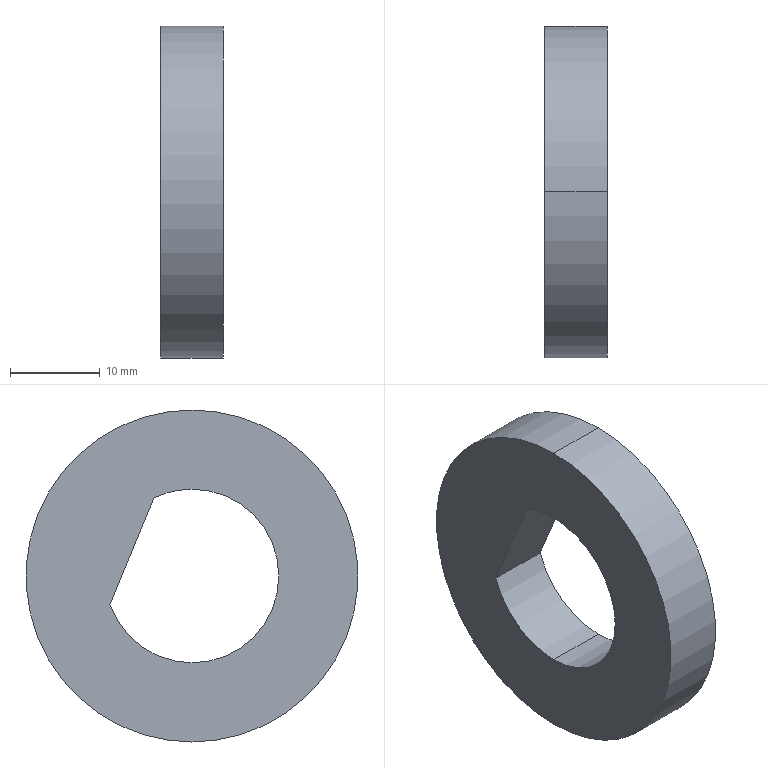Part | STEP file | Previa 01.sldasm-Part-11_Valor predeterminado | 1 solid | 8 faces | box 7 x 37.038 x 37.038 mm | volume 5630 mm3 | cylinder 5 | plane 3 | commonest cylinder face diameters 19.36 x3 37.038 x2
STEP:
#1=CARTESIAN_POINT('',(0.,0.,0.));
#2=DIRECTION('',(0.,0.,1.));
#3=DIRECTION('',(1.,0.,0.));
#4=AXIS2_PLACEMENT_3D('',#1,#2,#3);
#5=CARTESIAN_POINT('',(5.341,0.,-9.68));
#6=VERTEX_POINT('',#5);
#7=CARTESIAN_POINT('',(12.341,0.,-9.68));
#8=VERTEX_POINT('',#7);
#9=CARTESIAN_POINT('',(5.341,0.,-9.68));
#10=DIRECTION('',(1.,0.,0.));
#11=VECTOR('',#10,1.);
#12=LINE('',#9,#11);
#13=CARTESIAN_POINT('',(5.341,0.,0.));
#14=DIRECTION('',(1.,0.,0.));
#15=DIRECTION('',(0.,0.,-1.));
#16=AXIS2_PLACEMENT_3D('',#13,#14,#15);
#17=CYLINDRICAL_SURFACE('',#16,9.68);
#18=CARTESIAN_POINT('',(6.283,0.));
#19=DIRECTION('',(0.,1.));
#20=VECTOR('',#19,1.);
#21=LINE('',#18,#20);
#22=(GEOMETRIC_REPRESENTATION_CONTEXT(2)PARAMETRIC_REPRESENTATION_CONTEXT()REPRESENTATION_CONTEXT('',''));
#23=DEFINITIONAL_REPRESENTATION('',(#21),#22);
#24=PCURVE('',#17,#23);
#25=CARTESIAN_POINT('',(5.341,0.,0.));
#26=DIRECTION('',(1.,0.,0.));
#27=DIRECTION('',(0.,0.,-1.));
#28=AXIS2_PLACEMENT_3D('',#25,#26,#27);
#29=CYLINDRICAL_SURFACE('',#28,9.68);
#30=CARTESIAN_POINT('',(0.,0.));
#31=DIRECTION('',(0.,1.));
#32=VECTOR('',#31,1.);
#33=LINE('',#30,#32);
#34=(GEOMETRIC_REPRESENTATION_CONTEXT(2)PARAMETRIC_REPRESENTATION_CONTEXT()REPRESENTATION_CONTEXT('',''));
#35=DEFINITIONAL_REPRESENTATION('',(#33),#34);
#36=PCURVE('',#29,#35);
#37=SURFACE_CURVE('',#12,(#24,#36),.PCURVE_S1.);
#38=EDGE_CURVE('',#6,#8,#37,.T.);
#39=ORIENTED_EDGE('',*,*,#38,.T.);
#40=CARTESIAN_POINT('',(12.341,0.,9.68));
#41=VERTEX_POINT('',#40);
#42=CARTESIAN_POINT('',(12.341,0.,0.));
#43=DIRECTION('',(-1.,0.,0.));
#44=DIRECTION('',(0.,0.,-1.));
#45=AXIS2_PLACEMENT_3D('',#42,#43,#44);
#46=CIRCLE('',#45,9.68);
#47=CARTESIAN_POINT('',(6.283,7.));
#48=DIRECTION('',(-1.,0.));
#49=VECTOR('',#48,1.);
#50=LINE('',#47,#49);
#51=(GEOMETRIC_REPRESENTATION_CONTEXT(2)PARAMETRIC_REPRESENTATION_CONTEXT()REPRESENTATION_CONTEXT('',''));
#52=DEFINITIONAL_REPRESENTATION('',(#50),#51);
#53=PCURVE('',#17,#52);
#54=CARTESIAN_POINT('',(12.341,0.,0.));
#55=DIRECTION('',(-1.,0.,0.));
#56=DIRECTION('',(0.,0.,1.));
#57=AXIS2_PLACEMENT_3D('',#54,#55,#56);
#58=PLANE('',#57);
#59=CARTESIAN_POINT('',(0.,0.));
#60=DIRECTION('',(-1.,0.));
#61=AXIS2_PLACEMENT_2D('',#59,#60);
#62=CIRCLE('',#61,9.68);
#63=(GEOMETRIC_REPRESENTATION_CONTEXT(2)PARAMETRIC_REPRESENTATION_CONTEXT()REPRESENTATION_CONTEXT('',''));
#64=DEFINITIONAL_REPRESENTATION('',(#62),#63);
#65=PCURVE('',#58,#64);
#66=SURFACE_CURVE('',#46,(#53,#65),.PCURVE_S1.);
#67=EDGE_CURVE('',#8,#41,#66,.T.);
#68=ORIENTED_EDGE('',*,*,#67,.T.);
#69=CARTESIAN_POINT('',(5.341,0.,9.68));
#70=VERTEX_POINT('',#69);
#71=CARTESIAN_POINT('',(5.341,0.,9.68));
#72=DIRECTION('',(1.,0.,0.));
#73=VECTOR('',#72,1.);
#74=LINE('',#71,#73);
#75=CARTESIAN_POINT('',(3.142,0.));
#76=DIRECTION('',(0.,1.));
#77=VECTOR('',#76,1.);
#78=LINE('',#75,#77);
#79=(GEOMETRIC_REPRESENTATION_CONTEXT(2)PARAMETRIC_REPRESENTATION_CONTEXT()REPRESENTATION_CONTEXT('',''));
#80=DEFINITIONAL_REPRESENTATION('',(#78),#79);
#81=PCURVE('',#17,#80);
#82=CARTESIAN_POINT('',(5.341,0.,0.));
#83=DIRECTION('',(1.,0.,0.));
#84=DIRECTION('',(0.,0.,-1.));
#85=AXIS2_PLACEMENT_3D('',#82,#83,#84);
#86=CYLINDRICAL_SURFACE('',#85,9.68);
#87=CARTESIAN_POINT('',(3.142,0.));
#88=DIRECTION('',(0.,1.));
#89=VECTOR('',#88,1.);
#90=LINE('',#87,#89);
#91=(GEOMETRIC_REPRESENTATION_CONTEXT(2)PARAMETRIC_REPRESENTATION_CONTEXT()REPRESENTATION_CONTEXT('',''));
#92=DEFINITIONAL_REPRESENTATION('',(#90),#91);
#93=PCURVE('',#86,#92);
#94=SURFACE_CURVE('',#74,(#81,#93),.PCURVE_S1.);
#95=EDGE_CURVE('',#70,#41,#94,.T.);
#96=ORIENTED_EDGE('',*,*,#95,.F.);
#97=CARTESIAN_POINT('',(5.341,0.,0.));
#98=DIRECTION('',(-1.,0.,0.));
#99=DIRECTION('',(0.,0.,-1.));
#100=AXIS2_PLACEMENT_3D('',#97,#98,#99);
#101=CIRCLE('',#100,9.68);
#102=CARTESIAN_POINT('',(6.283,0.));
#103=DIRECTION('',(-1.,0.));
#104=VECTOR('',#103,1.);
#105=LINE('',#102,#104);
#106=(GEOMETRIC_REPRESENTATION_CONTEXT(2)PARAMETRIC_REPRESENTATION_CONTEXT()REPRESENTATION_CONTEXT('',''));
#107=DEFINITIONAL_REPRESENTATION('',(#105),#106);
#108=PCURVE('',#17,#107);
#109=CARTESIAN_POINT('',(5.341,0.,0.));
#110=DIRECTION('',(-1.,0.,0.));
#111=DIRECTION('',(0.,0.,1.));
#112=AXIS2_PLACEMENT_3D('',#109,#110,#111);
#113=PLANE('',#112);
#114=CARTESIAN_POINT('',(0.,0.));
#115=DIRECTION('',(-1.,0.));
#116=AXIS2_PLACEMENT_2D('',#114,#115);
#117=CIRCLE('',#116,9.68);
#118=(GEOMETRIC_REPRESENTATION_CONTEXT(2)PARAMETRIC_REPRESENTATION_CONTEXT()REPRESENTATION_CONTEXT('',''));
#119=DEFINITIONAL_REPRESENTATION('',(#117),#118);
#120=PCURVE('',#113,#119);
#121=SURFACE_CURVE('',#101,(#108,#120),.PCURVE_S1.);
#122=EDGE_CURVE('',#6,#70,#121,.T.);
#123=ORIENTED_EDGE('',*,*,#122,.F.);
#124=EDGE_LOOP('',(#39,#68,#96,#123));
#125=FACE_BOUND('',#124,.F.);
#126=ADVANCED_FACE('',(#125),#17,.F.);
#127=CARTESIAN_POINT('',(5.341,9.153,-3.149));
#128=VERTEX_POINT('',#127);
#129=CARTESIAN_POINT('',(12.341,9.153,-3.149));
#130=VERTEX_POINT('',#129);
#131=CARTESIAN_POINT('',(5.341,9.153,-3.149));
#132=DIRECTION('',(1.,0.,0.));
#133=VECTOR('',#132,1.);
#134=LINE('',#131,#133);
#135=CARTESIAN_POINT('',(1.239,0.));
#136=DIRECTION('',(0.,1.));
#137=VECTOR('',#136,1.);
#138=LINE('',#135,#137);
#139=(GEOMETRIC_REPRESENTATION_CONTEXT(2)PARAMETRIC_REPRESENTATION_CONTEXT()REPRESENTATION_CONTEXT('',''));
#140=DEFINITIONAL_REPRESENTATION('',(#138),#139);
#141=PCURVE('',#29,#140);
#142=CARTESIAN_POINT('',(5.341,4.269,8.688));
#143=DIRECTION('',(0.,-0.9244,-0.3814));
#144=DIRECTION('',(0.,0.3814,-0.9244));
#145=AXIS2_PLACEMENT_3D('',#142,#143,#144);
#146=PLANE('',#145);
#147=CARTESIAN_POINT('',(12.805,0.));
#148=DIRECTION('',(0.,1.));
#149=VECTOR('',#148,1.);
#150=LINE('',#147,#149);
#151=(GEOMETRIC_REPRESENTATION_CONTEXT(2)PARAMETRIC_REPRESENTATION_CONTEXT()REPRESENTATION_CONTEXT('',''));
#152=DEFINITIONAL_REPRESENTATION('',(#150),#151);
#153=PCURVE('',#146,#152);
#154=SURFACE_CURVE('',#134,(#141,#153),.PCURVE_S1.);
#155=EDGE_CURVE('',#128,#130,#154,.T.);
#156=ORIENTED_EDGE('',*,*,#155,.T.);
#157=CARTESIAN_POINT('',(12.341,0.,0.));
#158=DIRECTION('',(-1.,0.,0.));
#159=DIRECTION('',(0.,0.,-1.));
#160=AXIS2_PLACEMENT_3D('',#157,#158,#159);
#161=CIRCLE('',#160,9.68);
#162=CARTESIAN_POINT('',(6.283,7.));
#163=DIRECTION('',(-1.,0.));
#164=VECTOR('',#163,1.);
#165=LINE('',#162,#164);
#166=(GEOMETRIC_REPRESENTATION_CONTEXT(2)PARAMETRIC_REPRESENTATION_CONTEXT()REPRESENTATION_CONTEXT('',''));
#167=DEFINITIONAL_REPRESENTATION('',(#165),#166);
#168=PCURVE('',#29,#167);
#169=CARTESIAN_POINT('',(0.,0.));
#170=DIRECTION('',(-1.,0.));
#171=AXIS2_PLACEMENT_2D('',#169,#170);
#172=CIRCLE('',#171,9.68);
#173=(GEOMETRIC_REPRESENTATION_CONTEXT(2)PARAMETRIC_REPRESENTATION_CONTEXT()REPRESENTATION_CONTEXT('',''));
#174=DEFINITIONAL_REPRESENTATION('',(#172),#173);
#175=PCURVE('',#58,#174);
#176=SURFACE_CURVE('',#161,(#168,#175),.PCURVE_S1.);
#177=EDGE_CURVE('',#130,#8,#176,.T.);
#178=ORIENTED_EDGE('',*,*,#177,.T.);
#179=ORIENTED_EDGE('',*,*,#38,.F.);
#180=CARTESIAN_POINT('',(5.341,0.,0.));
#181=DIRECTION('',(-1.,0.,0.));
#182=DIRECTION('',(0.,0.,-1.));
#183=AXIS2_PLACEMENT_3D('',#180,#181,#182);
#184=CIRCLE('',#183,9.68);
#185=CARTESIAN_POINT('',(6.283,0.));
#186=DIRECTION('',(-1.,0.));
#187=VECTOR('',#186,1.);
#188=LINE('',#185,#187);
#189=(GEOMETRIC_REPRESENTATION_CONTEXT(2)PARAMETRIC_REPRESENTATION_CONTEXT()REPRESENTATION_CONTEXT('',''));
#190=DEFINITIONAL_REPRESENTATION('',(#188),#189);
#191=PCURVE('',#29,#190);
#192=CARTESIAN_POINT('',(0.,0.));
#193=DIRECTION('',(-1.,0.));
#194=AXIS2_PLACEMENT_2D('',#192,#193);
#195=CIRCLE('',#194,9.68);
#196=(GEOMETRIC_REPRESENTATION_CONTEXT(2)PARAMETRIC_REPRESENTATION_CONTEXT()REPRESENTATION_CONTEXT('',''));
#197=DEFINITIONAL_REPRESENTATION('',(#195),#196);
#198=PCURVE('',#113,#197);
#199=SURFACE_CURVE('',#184,(#191,#198),.PCURVE_S1.);
#200=EDGE_CURVE('',#128,#6,#199,.T.);
#201=ORIENTED_EDGE('',*,*,#200,.F.);
#202=EDGE_LOOP('',(#156,#178,#179,#201));
#203=FACE_BOUND('',#202,.F.);
#204=ADVANCED_FACE('',(#203),#29,.F.);
#205=CARTESIAN_POINT('',(5.341,0.,18.519));
#206=VERTEX_POINT('',#205);
#207=CARTESIAN_POINT('',(5.341,0.,-18.519));
#208=VERTEX_POINT('',#207);
#209=CARTESIAN_POINT('',(5.341,0.,0.));
#210=DIRECTION('',(-1.,0.,0.));
#211=DIRECTION('',(0.,0.,-1.));
#212=AXIS2_PLACEMENT_3D('',#209,#210,#211);
#213=CIRCLE('',#212,18.519);
#214=CARTESIAN_POINT('',(5.341,0.,0.));
#215=DIRECTION('',(1.,0.,0.));
#216=DIRECTION('',(0.,0.,-1.));
#217=AXIS2_PLACEMENT_3D('',#214,#215,#216);
#218=CYLINDRICAL_SURFACE('',#217,18.519);
#219=CARTESIAN_POINT('',(6.283,0.));
#220=DIRECTION('',(-1.,0.));
#221=VECTOR('',#220,1.);
#222=LINE('',#219,#221);
#223=(GEOMETRIC_REPRESENTATION_CONTEXT(2)PARAMETRIC_REPRESENTATION_CONTEXT()REPRESENTATION_CONTEXT('',''));
#224=DEFINITIONAL_REPRESENTATION('',(#222),#223);
#225=PCURVE('',#218,#224);
#226=CARTESIAN_POINT('',(0.,0.));
#227=DIRECTION('',(-1.,0.));
#228=AXIS2_PLACEMENT_2D('',#226,#227);
#229=CIRCLE('',#228,18.519);
#230=(GEOMETRIC_REPRESENTATION_CONTEXT(2)PARAMETRIC_REPRESENTATION_CONTEXT()REPRESENTATION_CONTEXT('',''));
#231=DEFINITIONAL_REPRESENTATION('',(#229),#230);
#232=PCURVE('',#113,#231);
#233=SURFACE_CURVE('',#213,(#225,#232),.PCURVE_S1.);
#234=EDGE_CURVE('',#206,#208,#233,.T.);
#235=ORIENTED_EDGE('',*,*,#234,.F.);
#236=CARTESIAN_POINT('',(12.341,0.,18.519));
#237=VERTEX_POINT('',#236);
#238=CARTESIAN_POINT('',(5.341,0.,18.519));
#239=DIRECTION('',(1.,0.,0.));
#240=VECTOR('',#239,1.);
#241=LINE('',#238,#240);
#242=CARTESIAN_POINT('',(3.142,0.));
#243=DIRECTION('',(0.,1.));
#244=VECTOR('',#243,1.);
#245=LINE('',#242,#244);
#246=(GEOMETRIC_REPRESENTATION_CONTEXT(2)PARAMETRIC_REPRESENTATION_CONTEXT()REPRESENTATION_CONTEXT('',''));
#247=DEFINITIONAL_REPRESENTATION('',(#245),#246);
#248=PCURVE('',#218,#247);
#249=CARTESIAN_POINT('',(5.341,0.,0.));
#250=DIRECTION('',(1.,0.,0.));
#251=DIRECTION('',(0.,0.,-1.));
#252=AXIS2_PLACEMENT_3D('',#249,#250,#251);
#253=CYLINDRICAL_SURFACE('',#252,18.519);
#254=CARTESIAN_POINT('',(3.142,0.));
#255=DIRECTION('',(0.,1.));
#256=VECTOR('',#255,1.);
#257=LINE('',#254,#256);
#258=(GEOMETRIC_REPRESENTATION_CONTEXT(2)PARAMETRIC_REPRESENTATION_CONTEXT()REPRESENTATION_CONTEXT('',''));
#259=DEFINITIONAL_REPRESENTATION('',(#257),#258);
#260=PCURVE('',#253,#259);
#261=SURFACE_CURVE('',#241,(#248,#260),.PCURVE_S1.);
#262=EDGE_CURVE('',#206,#237,#261,.T.);
#263=ORIENTED_EDGE('',*,*,#262,.T.);
#264=CARTESIAN_POINT('',(12.341,0.,-18.519));
#265=VERTEX_POINT('',#264);
#266=CARTESIAN_POINT('',(12.341,0.,0.));
#267=DIRECTION('',(-1.,0.,0.));
#268=DIRECTION('',(0.,0.,-1.));
#269=AXIS2_PLACEMENT_3D('',#266,#267,#268);
#270=CIRCLE('',#269,18.519);
#271=CARTESIAN_POINT('',(6.283,7.));
#272=DIRECTION('',(-1.,0.));
#273=VECTOR('',#272,1.);
#274=LINE('',#271,#273);
#275=(GEOMETRIC_REPRESENTATION_CONTEXT(2)PARAMETRIC_REPRESENTATION_CONTEXT()REPRESENTATION_CONTEXT('',''));
#276=DEFINITIONAL_REPRESENTATION('',(#274),#275);
#277=PCURVE('',#218,#276);
#278=CARTESIAN_POINT('',(0.,0.));
#279=DIRECTION('',(-1.,0.));
#280=AXIS2_PLACEMENT_2D('',#278,#279);
#281=CIRCLE('',#280,18.519);
#282=(GEOMETRIC_REPRESENTATION_CONTEXT(2)PARAMETRIC_REPRESENTATION_CONTEXT()REPRESENTATION_CONTEXT('',''));
#283=DEFINITIONAL_REPRESENTATION('',(#281),#282);
#284=PCURVE('',#58,#283);
#285=SURFACE_CURVE('',#270,(#277,#284),.PCURVE_S1.);
#286=EDGE_CURVE('',#237,#265,#285,.T.);
#287=ORIENTED_EDGE('',*,*,#286,.T.);
#288=CARTESIAN_POINT('',(5.341,0.,-18.519));
#289=DIRECTION('',(1.,0.,0.));
#290=VECTOR('',#289,1.);
#291=LINE('',#288,#290);
#292=CARTESIAN_POINT('',(0.,0.));
#293=DIRECTION('',(0.,1.));
#294=VECTOR('',#293,1.);
#295=LINE('',#292,#294);
#296=(GEOMETRIC_REPRESENTATION_CONTEXT(2)PARAMETRIC_REPRESENTATION_CONTEXT()REPRESENTATION_CONTEXT('',''));
#297=DEFINITIONAL_REPRESENTATION('',(#295),#296);
#298=PCURVE('',#218,#297);
#299=CARTESIAN_POINT('',(6.283,0.));
#300=DIRECTION('',(0.,1.));
#301=VECTOR('',#300,1.);
#302=LINE('',#299,#301);
#303=(GEOMETRIC_REPRESENTATION_CONTEXT(2)PARAMETRIC_REPRESENTATION_CONTEXT()REPRESENTATION_CONTEXT('',''));
#304=DEFINITIONAL_REPRESENTATION('',(#302),#303);
#305=PCURVE('',#253,#304);
#306=SURFACE_CURVE('',#291,(#298,#305),.PCURVE_S1.);
#307=EDGE_CURVE('',#208,#265,#306,.T.);
#308=ORIENTED_EDGE('',*,*,#307,.F.);
#309=EDGE_LOOP('',(#235,#263,#287,#308));
#310=FACE_BOUND('',#309,.T.);
#311=ADVANCED_FACE('',(#310),#218,.T.);
#312=CARTESIAN_POINT('',(12.341,4.269,8.688));
#313=VERTEX_POINT('',#312);
#314=CARTESIAN_POINT('',(12.341,4.269,8.688));
#315=DIRECTION('',(0.,0.3814,-0.9244));
#316=VECTOR('',#315,1.);
#317=LINE('',#314,#316);
#318=CARTESIAN_POINT('',(0.,7.));
#319=DIRECTION('',(1.,0.));
#320=VECTOR('',#319,1.);
#321=LINE('',#318,#320);
#322=(GEOMETRIC_REPRESENTATION_CONTEXT(2)PARAMETRIC_REPRESENTATION_CONTEXT()REPRESENTATION_CONTEXT('',''));
#323=DEFINITIONAL_REPRESENTATION('',(#321),#322);
#324=PCURVE('',#146,#323);
#325=CARTESIAN_POINT('',(8.688,4.269));
#326=DIRECTION('',(-0.9244,0.3814));
#327=VECTOR('',#326,1.);
#328=LINE('',#325,#327);
#329=(GEOMETRIC_REPRESENTATION_CONTEXT(2)PARAMETRIC_REPRESENTATION_CONTEXT()REPRESENTATION_CONTEXT('',''));
#330=DEFINITIONAL_REPRESENTATION('',(#328),#329);
#331=PCURVE('',#58,#330);
#332=SURFACE_CURVE('',#317,(#324,#331),.PCURVE_S1.);
#333=EDGE_CURVE('',#313,#130,#332,.T.);
#334=ORIENTED_EDGE('',*,*,#333,.F.);
#335=CARTESIAN_POINT('',(5.341,4.269,8.688));
#336=VERTEX_POINT('',#335);
#337=CARTESIAN_POINT('',(5.341,4.269,8.688));
#338=DIRECTION('',(1.,0.,0.));
#339=VECTOR('',#338,1.);
#340=LINE('',#337,#339);
#341=CARTESIAN_POINT('',(0.,0.));
#342=DIRECTION('',(0.,1.));
#343=VECTOR('',#342,1.);
#344=LINE('',#341,#343);
#345=(GEOMETRIC_REPRESENTATION_CONTEXT(2)PARAMETRIC_REPRESENTATION_CONTEXT()REPRESENTATION_CONTEXT('',''));
#346=DEFINITIONAL_REPRESENTATION('',(#344),#345);
#347=PCURVE('',#146,#346);
#348=CARTESIAN_POINT('',(2.685,0.));
#349=DIRECTION('',(0.,1.));
#350=VECTOR('',#349,1.);
#351=LINE('',#348,#350);
#352=(GEOMETRIC_REPRESENTATION_CONTEXT(2)PARAMETRIC_REPRESENTATION_CONTEXT()REPRESENTATION_CONTEXT('',''));
#353=DEFINITIONAL_REPRESENTATION('',(#351),#352);
#354=PCURVE('',#86,#353);
#355=SURFACE_CURVE('',#340,(#347,#354),.PCURVE_S1.);
#356=EDGE_CURVE('',#336,#313,#355,.T.);
#357=ORIENTED_EDGE('',*,*,#356,.F.);
#358=CARTESIAN_POINT('',(5.341,4.269,8.688));
#359=DIRECTION('',(0.,0.3814,-0.9244));
#360=VECTOR('',#359,1.);
#361=LINE('',#358,#360);
#362=CARTESIAN_POINT('',(0.,0.));
#363=DIRECTION('',(1.,0.));
#364=VECTOR('',#363,1.);
#365=LINE('',#362,#364);
#366=(GEOMETRIC_REPRESENTATION_CONTEXT(2)PARAMETRIC_REPRESENTATION_CONTEXT()REPRESENTATION_CONTEXT('',''));
#367=DEFINITIONAL_REPRESENTATION('',(#365),#366);
#368=PCURVE('',#146,#367);
#369=CARTESIAN_POINT('',(8.688,4.269));
#370=DIRECTION('',(-0.9244,0.3814));
#371=VECTOR('',#370,1.);
#372=LINE('',#369,#371);
#373=(GEOMETRIC_REPRESENTATION_CONTEXT(2)PARAMETRIC_REPRESENTATION_CONTEXT()REPRESENTATION_CONTEXT('',''));
#374=DEFINITIONAL_REPRESENTATION('',(#372),#373);
#375=PCURVE('',#113,#374);
#376=SURFACE_CURVE('',#361,(#368,#375),.PCURVE_S1.);
#377=EDGE_CURVE('',#336,#128,#376,.T.);
#378=ORIENTED_EDGE('',*,*,#377,.T.);
#379=ORIENTED_EDGE('',*,*,#155,.T.);
#380=EDGE_LOOP('',(#334,#357,#378,#379));
#381=FACE_BOUND('',#380,.T.);
#382=ADVANCED_FACE('',(#381),#146,.T.);
#383=ORIENTED_EDGE('',*,*,#262,.F.);
#384=CARTESIAN_POINT('',(5.341,0.,0.));
#385=DIRECTION('',(-1.,0.,0.));
#386=DIRECTION('',(0.,0.,-1.));
#387=AXIS2_PLACEMENT_3D('',#384,#385,#386);
#388=CIRCLE('',#387,18.519);
#389=CARTESIAN_POINT('',(6.283,0.));
#390=DIRECTION('',(-1.,0.));
#391=VECTOR('',#390,1.);
#392=LINE('',#389,#391);
#393=(GEOMETRIC_REPRESENTATION_CONTEXT(2)PARAMETRIC_REPRESENTATION_CONTEXT()REPRESENTATION_CONTEXT('',''));
#394=DEFINITIONAL_REPRESENTATION('',(#392),#393);
#395=PCURVE('',#253,#394);
#396=CARTESIAN_POINT('',(0.,0.));
#397=DIRECTION('',(-1.,0.));
#398=AXIS2_PLACEMENT_2D('',#396,#397);
#399=CIRCLE('',#398,18.519);
#400=(GEOMETRIC_REPRESENTATION_CONTEXT(2)PARAMETRIC_REPRESENTATION_CONTEXT()REPRESENTATION_CONTEXT('',''));
#401=DEFINITIONAL_REPRESENTATION('',(#399),#400);
#402=PCURVE('',#113,#401);
#403=SURFACE_CURVE('',#388,(#395,#402),.PCURVE_S1.);
#404=EDGE_CURVE('',#208,#206,#403,.T.);
#405=ORIENTED_EDGE('',*,*,#404,.F.);
#406=ORIENTED_EDGE('',*,*,#307,.T.);
#407=CARTESIAN_POINT('',(12.341,0.,0.));
#408=DIRECTION('',(-1.,0.,0.));
#409=DIRECTION('',(0.,0.,-1.));
#410=AXIS2_PLACEMENT_3D('',#407,#408,#409);
#411=CIRCLE('',#410,18.519);
#412=CARTESIAN_POINT('',(6.283,7.));
#413=DIRECTION('',(-1.,0.));
#414=VECTOR('',#413,1.);
#415=LINE('',#412,#414);
#416=(GEOMETRIC_REPRESENTATION_CONTEXT(2)PARAMETRIC_REPRESENTATION_CONTEXT()REPRESENTATION_CONTEXT('',''));
#417=DEFINITIONAL_REPRESENTATION('',(#415),#416);
#418=PCURVE('',#253,#417);
#419=CARTESIAN_POINT('',(0.,0.));
#420=DIRECTION('',(-1.,0.));
#421=AXIS2_PLACEMENT_2D('',#419,#420);
#422=CIRCLE('',#421,18.519);
#423=(GEOMETRIC_REPRESENTATION_CONTEXT(2)PARAMETRIC_REPRESENTATION_CONTEXT()REPRESENTATION_CONTEXT('',''));
#424=DEFINITIONAL_REPRESENTATION('',(#422),#423);
#425=PCURVE('',#58,#424);
#426=SURFACE_CURVE('',#411,(#418,#425),.PCURVE_S1.);
#427=EDGE_CURVE('',#265,#237,#426,.T.);
#428=ORIENTED_EDGE('',*,*,#427,.T.);
#429=EDGE_LOOP('',(#383,#405,#406,#428));
#430=FACE_BOUND('',#429,.T.);
#431=ADVANCED_FACE('',(#430),#253,.T.);
#432=CARTESIAN_POINT('',(12.341,0.,0.));
#433=DIRECTION('',(-1.,0.,0.));
#434=DIRECTION('',(0.,0.,-1.));
#435=AXIS2_PLACEMENT_3D('',#432,#433,#434);
#436=CIRCLE('',#435,9.68);
#437=CARTESIAN_POINT('',(6.283,7.));
#438=DIRECTION('',(-1.,0.));
#439=VECTOR('',#438,1.);
#440=LINE('',#437,#439);
#441=(GEOMETRIC_REPRESENTATION_CONTEXT(2)PARAMETRIC_REPRESENTATION_CONTEXT()REPRESENTATION_CONTEXT('',''));
#442=DEFINITIONAL_REPRESENTATION('',(#440),#441);
#443=PCURVE('',#86,#442);
#444=CARTESIAN_POINT('',(0.,0.));
#445=DIRECTION('',(-1.,0.));
#446=AXIS2_PLACEMENT_2D('',#444,#445);
#447=CIRCLE('',#446,9.68);
#448=(GEOMETRIC_REPRESENTATION_CONTEXT(2)PARAMETRIC_REPRESENTATION_CONTEXT()REPRESENTATION_CONTEXT('',''));
#449=DEFINITIONAL_REPRESENTATION('',(#447),#448);
#450=PCURVE('',#58,#449);
#451=SURFACE_CURVE('',#436,(#443,#450),.PCURVE_S1.);
#452=EDGE_CURVE('',#41,#313,#451,.T.);
#453=ORIENTED_EDGE('',*,*,#452,.T.);
#454=ORIENTED_EDGE('',*,*,#356,.F.);
#455=CARTESIAN_POINT('',(5.341,0.,0.));
#456=DIRECTION('',(-1.,0.,0.));
#457=DIRECTION('',(0.,0.,-1.));
#458=AXIS2_PLACEMENT_3D('',#455,#456,#457);
#459=CIRCLE('',#458,9.68);
#460=CARTESIAN_POINT('',(6.283,0.));
#461=DIRECTION('',(-1.,0.));
#462=VECTOR('',#461,1.);
#463=LINE('',#460,#462);
#464=(GEOMETRIC_REPRESENTATION_CONTEXT(2)PARAMETRIC_REPRESENTATION_CONTEXT()REPRESENTATION_CONTEXT('',''));
#465=DEFINITIONAL_REPRESENTATION('',(#463),#464);
#466=PCURVE('',#86,#465);
#467=CARTESIAN_POINT('',(0.,0.));
#468=DIRECTION('',(-1.,0.));
#469=AXIS2_PLACEMENT_2D('',#467,#468);
#470=CIRCLE('',#469,9.68);
#471=(GEOMETRIC_REPRESENTATION_CONTEXT(2)PARAMETRIC_REPRESENTATION_CONTEXT()REPRESENTATION_CONTEXT('',''));
#472=DEFINITIONAL_REPRESENTATION('',(#470),#471);
#473=PCURVE('',#113,#472);
#474=SURFACE_CURVE('',#459,(#466,#473),.PCURVE_S1.);
#475=EDGE_CURVE('',#70,#336,#474,.T.);
#476=ORIENTED_EDGE('',*,*,#475,.F.);
#477=ORIENTED_EDGE('',*,*,#95,.T.);
#478=EDGE_LOOP('',(#453,#454,#476,#477));
#479=FACE_BOUND('',#478,.F.);
#480=ADVANCED_FACE('',(#479),#86,.F.);
#481=ORIENTED_EDGE('',*,*,#404,.T.);
#482=ORIENTED_EDGE('',*,*,#234,.T.);
#483=EDGE_LOOP('',(#481,#482));
#484=FACE_BOUND('',#483,.T.);
#485=ORIENTED_EDGE('',*,*,#377,.F.);
#486=ORIENTED_EDGE('',*,*,#475,.F.);
#487=ORIENTED_EDGE('',*,*,#122,.F.);
#488=ORIENTED_EDGE('',*,*,#200,.F.);
#489=EDGE_LOOP('',(#485,#486,#487,#488));
#490=FACE_BOUND('',#489,.T.);
#491=ADVANCED_FACE('',(#484,#490),#113,.T.);
#492=ORIENTED_EDGE('',*,*,#427,.F.);
#493=ORIENTED_EDGE('',*,*,#286,.F.);
#494=EDGE_LOOP('',(#492,#493));
#495=FACE_BOUND('',#494,.T.);
#496=ORIENTED_EDGE('',*,*,#333,.T.);
#497=ORIENTED_EDGE('',*,*,#177,.T.);
#498=ORIENTED_EDGE('',*,*,#67,.T.);
#499=ORIENTED_EDGE('',*,*,#452,.T.);
#500=EDGE_LOOP('',(#496,#497,#498,#499));
#501=FACE_BOUND('',#500,.T.);
#502=ADVANCED_FACE('',(#495,#501),#58,.F.);
#503=CLOSED_SHELL('',(#126,#204,#311,#382,#431,#480,#491,#502));
#504=MANIFOLD_SOLID_BREP('',#503);
#505=(LENGTH_UNIT()NAMED_UNIT(*)SI_UNIT(.MILLI.,.METRE.));
#506=UNCERTAINTY_MEASURE_WITH_UNIT(LENGTH_MEASURE(0.0000001),#505,'','');
#507=(NAMED_UNIT(*)PLANE_ANGLE_UNIT()SI_UNIT($,.RADIAN.));
#508=(NAMED_UNIT(*)SI_UNIT($,.STERADIAN.)SOLID_ANGLE_UNIT());
#509=(GEOMETRIC_REPRESENTATION_CONTEXT(3)GLOBAL_UNCERTAINTY_ASSIGNED_CONTEXT((#506))GLOBAL_UNIT_ASSIGNED_CONTEXT((#505,#507,#508))REPRESENTATION_CONTEXT('',''));
#510=ADVANCED_BREP_SHAPE_REPRESENTATION('',(#4,#504),#509);